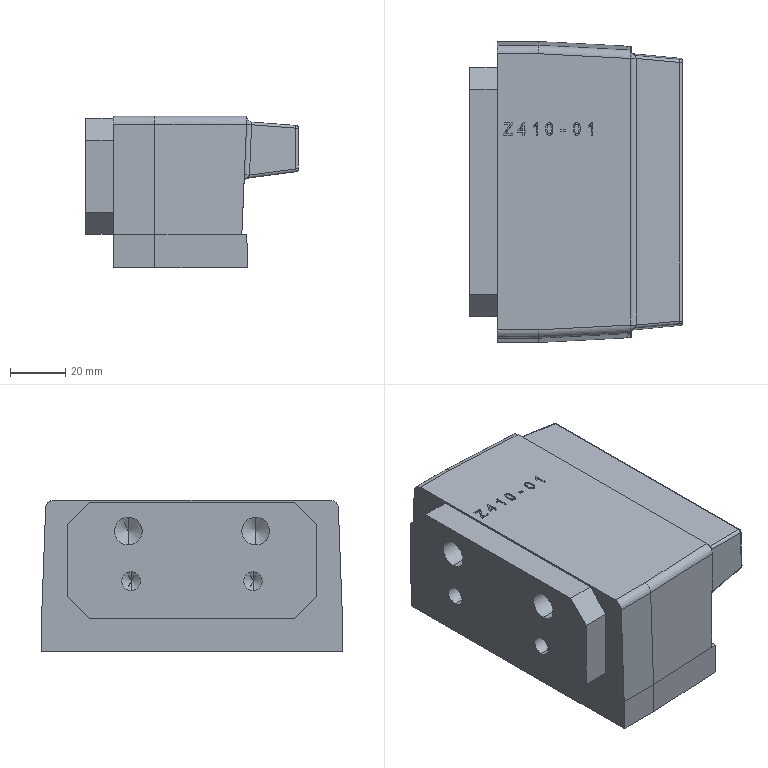Part | Creo | 1 solid | 178 faces | box 76.806 x 108.581 x 54.665 mm | volume 333496 mm3 | plane 76 | other 57 | cylinder 25 | cone 12 | spline 4 | sphere 4 | commonest cylinder face diameters 2.009 x8 4.018 x4 6 x4 6.7 x4 10 x4 60.776 x1